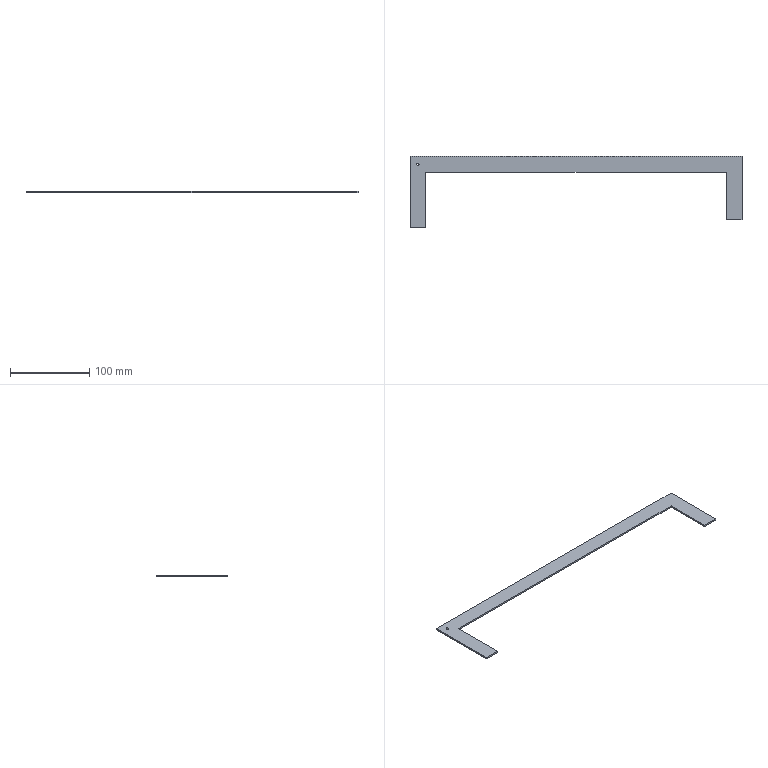Part | STEP file | Trunking Spacer Plate 2 | 1 solid | 12 faces | box 420 x 90 x 2 mm | volume 21986 mm3 | plane 10 | cylinder 2 | commonest cylinder face diameters 3 x2
STEP:
#1=CARTESIAN_POINT('',(1021.716,-891.567,-2.));
#2=VERTEX_POINT('',#1);
#3=CARTESIAN_POINT('',(1018.716,-891.567,-2.));
#4=VERTEX_POINT('',#3);
#5=CARTESIAN_POINT('',(1020.216,-891.567,-2.));
#6=DIRECTION('',(0.,0.,-1.));
#7=DIRECTION('',(1.,0.,0.));
#8=AXIS2_PLACEMENT_3D('',#5,#6,#7);
#9=CIRCLE('',#8,1.5);
#10=EDGE_CURVE('',#2,#4,#9,.T.);
#11=ORIENTED_EDGE('',*,*,#10,.T.);
#12=CARTESIAN_POINT('',(1018.716,-891.567,0.));
#13=VERTEX_POINT('',#12);
#14=CARTESIAN_POINT('',(1018.716,-891.567,-2.));
#15=DIRECTION('',(0.,0.,1.));
#16=VECTOR('',#15,1000.);
#17=LINE('',#14,#16);
#18=EDGE_CURVE('',#4,#13,#17,.T.);
#19=ORIENTED_EDGE('',*,*,#18,.T.);
#20=CARTESIAN_POINT('',(1021.716,-891.567,0.));
#21=VERTEX_POINT('',#20);
#22=CARTESIAN_POINT('',(1020.216,-891.567,0.));
#23=DIRECTION('',(0.,0.,-1.));
#24=DIRECTION('',(1.,0.,0.));
#25=AXIS2_PLACEMENT_3D('',#22,#23,#24);
#26=CIRCLE('',#25,1.5);
#27=EDGE_CURVE('',#21,#13,#26,.T.);
#28=ORIENTED_EDGE('',*,*,#27,.F.);
#29=CARTESIAN_POINT('',(1021.716,-891.567,-2.));
#30=DIRECTION('',(0.,0.,1.));
#31=VECTOR('',#30,1000.);
#32=LINE('',#29,#31);
#33=EDGE_CURVE('',#2,#21,#32,.T.);
#34=ORIENTED_EDGE('',*,*,#33,.F.);
#35=EDGE_LOOP('',(#11,#19,#28,#34));
#36=FACE_OUTER_BOUND('',#35,.T.);
#37=CARTESIAN_POINT('',(1020.216,-891.567,-2.));
#38=DIRECTION('',(0.,0.,1.));
#39=DIRECTION('',(1.,0.,0.));
#40=AXIS2_PLACEMENT_3D('',#37,#38,#39);
#41=CYLINDRICAL_SURFACE('',#40,1.5);
#42=ADVANCED_FACE('',(#36),#41,.F.);
#43=ORIENTED_EDGE('',*,*,#10,.F.);
#44=CARTESIAN_POINT('',(1020.216,-891.567,-2.));
#45=DIRECTION('',(0.,0.,-1.));
#46=DIRECTION('',(1.,0.,0.));
#47=AXIS2_PLACEMENT_3D('',#44,#45,#46);
#48=CIRCLE('',#47,1.5);
#49=EDGE_CURVE('',#4,#2,#48,.T.);
#50=ORIENTED_EDGE('',*,*,#49,.F.);
#51=EDGE_LOOP('',(#43,#50));
#52=FACE_BOUND('',#51,.T.);
#53=CARTESIAN_POINT('',(1410.216,-961.567,-2.));
#54=VERTEX_POINT('',#53);
#55=CARTESIAN_POINT('',(1430.216,-961.567,-2.));
#56=VERTEX_POINT('',#55);
#57=CARTESIAN_POINT('',(0.,-961.567,-2.));
#58=DIRECTION('',(1.,0.,0.));
#59=VECTOR('',#58,1000.);
#60=LINE('',#57,#59);
#61=EDGE_CURVE('',#54,#56,#60,.T.);
#62=ORIENTED_EDGE('',*,*,#61,.F.);
#63=CARTESIAN_POINT('',(1410.216,-901.567,-2.));
#64=VERTEX_POINT('',#63);
#65=CARTESIAN_POINT('',(1410.216,0.,-2.));
#66=DIRECTION('',(0.,-1.,0.));
#67=VECTOR('',#66,1000.);
#68=LINE('',#65,#67);
#69=EDGE_CURVE('',#64,#54,#68,.T.);
#70=ORIENTED_EDGE('',*,*,#69,.F.);
#71=CARTESIAN_POINT('',(1030.216,-901.567,-2.));
#72=VERTEX_POINT('',#71);
#73=CARTESIAN_POINT('',(0.,-901.567,-2.));
#74=DIRECTION('',(1.,0.,0.));
#75=VECTOR('',#74,1000.);
#76=LINE('',#73,#75);
#77=EDGE_CURVE('',#72,#64,#76,.T.);
#78=ORIENTED_EDGE('',*,*,#77,.F.);
#79=CARTESIAN_POINT('',(1030.216,-971.567,-2.));
#80=VERTEX_POINT('',#79);
#81=CARTESIAN_POINT('',(1030.216,0.,-2.));
#82=DIRECTION('',(0.,1.,0.));
#83=VECTOR('',#82,1000.);
#84=LINE('',#81,#83);
#85=EDGE_CURVE('',#80,#72,#84,.T.);
#86=ORIENTED_EDGE('',*,*,#85,.F.);
#87=CARTESIAN_POINT('',(1010.216,-971.567,-2.));
#88=VERTEX_POINT('',#87);
#89=CARTESIAN_POINT('',(0.,-971.567,-2.));
#90=DIRECTION('',(1.,0.,0.));
#91=VECTOR('',#90,1000.);
#92=LINE('',#89,#91);
#93=EDGE_CURVE('',#88,#80,#92,.T.);
#94=ORIENTED_EDGE('',*,*,#93,.F.);
#95=CARTESIAN_POINT('',(1010.216,-881.567,-2.));
#96=VERTEX_POINT('',#95);
#97=CARTESIAN_POINT('',(1010.216,0.,-2.));
#98=DIRECTION('',(0.,-1.,0.));
#99=VECTOR('',#98,1000.);
#100=LINE('',#97,#99);
#101=EDGE_CURVE('',#96,#88,#100,.T.);
#102=ORIENTED_EDGE('',*,*,#101,.F.);
#103=CARTESIAN_POINT('',(1430.216,-881.567,-2.));
#104=VERTEX_POINT('',#103);
#105=CARTESIAN_POINT('',(0.,-881.567,-2.));
#106=DIRECTION('',(-1.,0.,0.));
#107=VECTOR('',#106,1000.);
#108=LINE('',#105,#107);
#109=EDGE_CURVE('',#104,#96,#108,.T.);
#110=ORIENTED_EDGE('',*,*,#109,.F.);
#111=CARTESIAN_POINT('',(1430.216,0.,-2.));
#112=DIRECTION('',(0.,1.,0.));
#113=VECTOR('',#112,1000.);
#114=LINE('',#111,#113);
#115=EDGE_CURVE('',#56,#104,#114,.T.);
#116=ORIENTED_EDGE('',*,*,#115,.F.);
#117=EDGE_LOOP('',(#62,#70,#78,#86,#94,#102,#110,#116));
#118=FACE_OUTER_BOUND('',#117,.T.);
#119=CARTESIAN_POINT('',(0.,0.,-2.));
#120=DIRECTION('',(0.,0.,1.));
#121=DIRECTION('',(1.,0.,0.));
#122=AXIS2_PLACEMENT_3D('',#119,#120,#121);
#123=PLANE('',#122);
#124=ADVANCED_FACE('',(#52,#118),#123,.F.);
#125=ORIENTED_EDGE('',*,*,#18,.F.);
#126=ORIENTED_EDGE('',*,*,#49,.T.);
#127=ORIENTED_EDGE('',*,*,#33,.T.);
#128=CARTESIAN_POINT('',(1020.216,-891.567,0.));
#129=DIRECTION('',(0.,0.,-1.));
#130=DIRECTION('',(1.,0.,0.));
#131=AXIS2_PLACEMENT_3D('',#128,#129,#130);
#132=CIRCLE('',#131,1.5);
#133=EDGE_CURVE('',#13,#21,#132,.T.);
#134=ORIENTED_EDGE('',*,*,#133,.F.);
#135=EDGE_LOOP('',(#125,#126,#127,#134));
#136=FACE_OUTER_BOUND('',#135,.T.);
#137=CARTESIAN_POINT('',(1020.216,-891.567,-2.));
#138=DIRECTION('',(0.,0.,1.));
#139=DIRECTION('',(1.,0.,0.));
#140=AXIS2_PLACEMENT_3D('',#137,#138,#139);
#141=CYLINDRICAL_SURFACE('',#140,1.5);
#142=ADVANCED_FACE('',(#136),#141,.F.);
#143=CARTESIAN_POINT('',(1430.216,-881.567,0.));
#144=VERTEX_POINT('',#143);
#145=CARTESIAN_POINT('',(1430.216,-881.567,-2.));
#146=DIRECTION('',(0.,0.,1.));
#147=VECTOR('',#146,1000.);
#148=LINE('',#145,#147);
#149=EDGE_CURVE('',#104,#144,#148,.T.);
#150=ORIENTED_EDGE('',*,*,#149,.T.);
#151=CARTESIAN_POINT('',(1430.216,-961.567,0.));
#152=VERTEX_POINT('',#151);
#153=CARTESIAN_POINT('',(1430.216,-881.567,0.));
#154=DIRECTION('',(0.,-1.,0.));
#155=VECTOR('',#154,1000.);
#156=LINE('',#153,#155);
#157=EDGE_CURVE('',#144,#152,#156,.T.);
#158=ORIENTED_EDGE('',*,*,#157,.T.);
#159=CARTESIAN_POINT('',(1430.216,-961.567,-2.));
#160=DIRECTION('',(0.,0.,-1.));
#161=VECTOR('',#160,1000.);
#162=LINE('',#159,#161);
#163=EDGE_CURVE('',#152,#56,#162,.T.);
#164=ORIENTED_EDGE('',*,*,#163,.T.);
#165=ORIENTED_EDGE('',*,*,#115,.T.);
#166=EDGE_LOOP('',(#150,#158,#164,#165));
#167=FACE_OUTER_BOUND('',#166,.T.);
#168=CARTESIAN_POINT('',(1430.216,-881.567,-2.));
#169=DIRECTION('',(1.,0.,0.));
#170=DIRECTION('',(0.,1.,0.));
#171=AXIS2_PLACEMENT_3D('',#168,#169,#170);
#172=PLANE('',#171);
#173=ADVANCED_FACE('',(#167),#172,.T.);
#174=CARTESIAN_POINT('',(1410.216,-961.567,0.));
#175=VERTEX_POINT('',#174);
#176=CARTESIAN_POINT('',(1010.216,-961.567,0.));
#177=DIRECTION('',(1.,0.,0.));
#178=VECTOR('',#177,1000.);
#179=LINE('',#176,#178);
#180=EDGE_CURVE('',#175,#152,#179,.T.);
#181=ORIENTED_EDGE('',*,*,#180,.F.);
#182=CARTESIAN_POINT('',(1410.216,-961.567,-10.));
#183=DIRECTION('',(0.,0.,1.));
#184=VECTOR('',#183,1000.);
#185=LINE('',#182,#184);
#186=EDGE_CURVE('',#54,#175,#185,.T.);
#187=ORIENTED_EDGE('',*,*,#186,.F.);
#188=ORIENTED_EDGE('',*,*,#61,.T.);
#189=ORIENTED_EDGE('',*,*,#163,.F.);
#190=EDGE_LOOP('',(#181,#187,#188,#189));
#191=FACE_OUTER_BOUND('',#190,.T.);
#192=CARTESIAN_POINT('',(1010.216,-961.567,-10.));
#193=DIRECTION('',(0.,1.,0.));
#194=DIRECTION('',(0.,0.,1.));
#195=AXIS2_PLACEMENT_3D('',#192,#193,#194);
#196=PLANE('',#195);
#197=ADVANCED_FACE('',(#191),#196,.F.);
#198=ORIENTED_EDGE('',*,*,#186,.T.);
#199=CARTESIAN_POINT('',(1410.216,-901.567,0.));
#200=VERTEX_POINT('',#199);
#201=CARTESIAN_POINT('',(1410.216,-901.567,0.));
#202=DIRECTION('',(0.,-1.,0.));
#203=VECTOR('',#202,1000.);
#204=LINE('',#201,#203);
#205=EDGE_CURVE('',#200,#175,#204,.T.);
#206=ORIENTED_EDGE('',*,*,#205,.F.);
#207=CARTESIAN_POINT('',(1410.216,-901.567,-2.));
#208=DIRECTION('',(0.,0.,1.));
#209=VECTOR('',#208,1000.);
#210=LINE('',#207,#209);
#211=EDGE_CURVE('',#64,#200,#210,.T.);
#212=ORIENTED_EDGE('',*,*,#211,.F.);
#213=ORIENTED_EDGE('',*,*,#69,.T.);
#214=EDGE_LOOP('',(#198,#206,#212,#213));
#215=FACE_OUTER_BOUND('',#214,.T.);
#216=CARTESIAN_POINT('',(1410.216,-901.567,-2.));
#217=DIRECTION('',(1.,0.,0.));
#218=DIRECTION('',(0.,0.,-1.));
#219=AXIS2_PLACEMENT_3D('',#216,#217,#218);
#220=PLANE('',#219);
#221=ADVANCED_FACE('',(#215),#220,.F.);
#222=CARTESIAN_POINT('',(1030.216,-901.567,0.));
#223=VERTEX_POINT('',#222);
#224=CARTESIAN_POINT('',(1030.216,-901.567,-2.));
#225=DIRECTION('',(0.,0.,1.));
#226=VECTOR('',#225,1000.);
#227=LINE('',#224,#226);
#228=EDGE_CURVE('',#72,#223,#227,.T.);
#229=ORIENTED_EDGE('',*,*,#228,.F.);
#230=ORIENTED_EDGE('',*,*,#77,.T.);
#231=ORIENTED_EDGE('',*,*,#211,.T.);
#232=CARTESIAN_POINT('',(1030.216,-901.567,0.));
#233=DIRECTION('',(1.,0.,0.));
#234=VECTOR('',#233,1000.);
#235=LINE('',#232,#234);
#236=EDGE_CURVE('',#223,#200,#235,.T.);
#237=ORIENTED_EDGE('',*,*,#236,.F.);
#238=EDGE_LOOP('',(#229,#230,#231,#237));
#239=FACE_OUTER_BOUND('',#238,.T.);
#240=CARTESIAN_POINT('',(1030.216,-901.567,-2.));
#241=DIRECTION('',(0.,1.,0.));
#242=DIRECTION('',(0.,0.,1.));
#243=AXIS2_PLACEMENT_3D('',#240,#241,#242);
#244=PLANE('',#243);
#245=ADVANCED_FACE('',(#239),#244,.F.);
#246=CARTESIAN_POINT('',(1030.216,-971.567,0.));
#247=VERTEX_POINT('',#246);
#248=CARTESIAN_POINT('',(1030.216,-971.567,-2.));
#249=DIRECTION('',(0.,0.,1.));
#250=VECTOR('',#249,1000.);
#251=LINE('',#248,#250);
#252=EDGE_CURVE('',#80,#247,#251,.T.);
#253=ORIENTED_EDGE('',*,*,#252,.F.);
#254=ORIENTED_EDGE('',*,*,#85,.T.);
#255=ORIENTED_EDGE('',*,*,#228,.T.);
#256=CARTESIAN_POINT('',(1030.216,-901.567,0.));
#257=DIRECTION('',(0.,1.,0.));
#258=VECTOR('',#257,1000.);
#259=LINE('',#256,#258);
#260=EDGE_CURVE('',#247,#223,#259,.T.);
#261=ORIENTED_EDGE('',*,*,#260,.F.);
#262=EDGE_LOOP('',(#253,#254,#255,#261));
#263=FACE_OUTER_BOUND('',#262,.T.);
#264=CARTESIAN_POINT('',(1030.216,-901.567,-2.));
#265=DIRECTION('',(-1.,0.,0.));
#266=DIRECTION('',(0.,0.,1.));
#267=AXIS2_PLACEMENT_3D('',#264,#265,#266);
#268=PLANE('',#267);
#269=ADVANCED_FACE('',(#263),#268,.F.);
#270=CARTESIAN_POINT('',(1010.216,-971.567,0.));
#271=VERTEX_POINT('',#270);
#272=CARTESIAN_POINT('',(0.,-971.567,0.));
#273=DIRECTION('',(-1.,0.,0.));
#274=VECTOR('',#273,1000.);
#275=LINE('',#272,#274);
#276=EDGE_CURVE('',#247,#271,#275,.T.);
#277=ORIENTED_EDGE('',*,*,#276,.T.);
#278=CARTESIAN_POINT('',(1010.216,-971.567,0.));
#279=DIRECTION('',(0.,0.,-1.));
#280=VECTOR('',#279,1000.);
#281=LINE('',#278,#280);
#282=EDGE_CURVE('',#271,#88,#281,.T.);
#283=ORIENTED_EDGE('',*,*,#282,.T.);
#284=ORIENTED_EDGE('',*,*,#93,.T.);
#285=ORIENTED_EDGE('',*,*,#252,.T.);
#286=EDGE_LOOP('',(#277,#283,#284,#285));
#287=FACE_OUTER_BOUND('',#286,.T.);
#288=CARTESIAN_POINT('',(0.,-971.567,0.));
#289=DIRECTION('',(0.,-1.,0.));
#290=DIRECTION('',(0.,0.,-1.));
#291=AXIS2_PLACEMENT_3D('',#288,#289,#290);
#292=PLANE('',#291);
#293=ADVANCED_FACE('',(#287),#292,.T.);
#294=CARTESIAN_POINT('',(1010.216,-881.567,0.));
#295=VERTEX_POINT('',#294);
#296=CARTESIAN_POINT('',(1010.216,-881.567,0.));
#297=DIRECTION('',(0.,1.,0.));
#298=VECTOR('',#297,1000.);
#299=LINE('',#296,#298);
#300=EDGE_CURVE('',#271,#295,#299,.T.);
#301=ORIENTED_EDGE('',*,*,#300,.T.);
#302=CARTESIAN_POINT('',(1010.216,-881.567,-2.));
#303=DIRECTION('',(0.,0.,-1.));
#304=VECTOR('',#303,1000.);
#305=LINE('',#302,#304);
#306=EDGE_CURVE('',#295,#96,#305,.T.);
#307=ORIENTED_EDGE('',*,*,#306,.T.);
#308=ORIENTED_EDGE('',*,*,#101,.T.);
#309=ORIENTED_EDGE('',*,*,#282,.F.);
#310=EDGE_LOOP('',(#301,#307,#308,#309));
#311=FACE_OUTER_BOUND('',#310,.T.);
#312=CARTESIAN_POINT('',(1010.216,-881.567,-2.));
#313=DIRECTION('',(-1.,0.,0.));
#314=DIRECTION('',(0.,-1.,0.));
#315=AXIS2_PLACEMENT_3D('',#312,#313,#314);
#316=PLANE('',#315);
#317=ADVANCED_FACE('',(#311),#316,.T.);
#318=ORIENTED_EDGE('',*,*,#109,.T.);
#319=ORIENTED_EDGE('',*,*,#306,.F.);
#320=CARTESIAN_POINT('',(1010.216,-881.567,0.));
#321=DIRECTION('',(1.,0.,0.));
#322=VECTOR('',#321,1000.);
#323=LINE('',#320,#322);
#324=EDGE_CURVE('',#295,#144,#323,.T.);
#325=ORIENTED_EDGE('',*,*,#324,.T.);
#326=ORIENTED_EDGE('',*,*,#149,.F.);
#327=EDGE_LOOP('',(#318,#319,#325,#326));
#328=FACE_OUTER_BOUND('',#327,.T.);
#329=CARTESIAN_POINT('',(1010.216,-881.567,-2.));
#330=DIRECTION('',(0.,1.,0.));
#331=DIRECTION('',(0.,0.,1.));
#332=AXIS2_PLACEMENT_3D('',#329,#330,#331);
#333=PLANE('',#332);
#334=ADVANCED_FACE('',(#328),#333,.T.);
#335=ORIENTED_EDGE('',*,*,#27,.T.);
#336=ORIENTED_EDGE('',*,*,#133,.T.);
#337=EDGE_LOOP('',(#335,#336));
#338=FACE_BOUND('',#337,.T.);
#339=ORIENTED_EDGE('',*,*,#236,.T.);
#340=ORIENTED_EDGE('',*,*,#205,.T.);
#341=ORIENTED_EDGE('',*,*,#180,.T.);
#342=ORIENTED_EDGE('',*,*,#157,.F.);
#343=ORIENTED_EDGE('',*,*,#324,.F.);
#344=ORIENTED_EDGE('',*,*,#300,.F.);
#345=ORIENTED_EDGE('',*,*,#276,.F.);
#346=ORIENTED_EDGE('',*,*,#260,.T.);
#347=EDGE_LOOP('',(#339,#340,#341,#342,#343,#344,#345,#346));
#348=FACE_OUTER_BOUND('',#347,.T.);
#349=CARTESIAN_POINT('',(0.,0.,0.));
#350=DIRECTION('',(0.,0.,1.));
#351=DIRECTION('',(1.,0.,0.));
#352=AXIS2_PLACEMENT_3D('',#349,#350,#351);
#353=PLANE('',#352);
#354=ADVANCED_FACE('',(#338,#348),#353,.T.);
#355=CLOSED_SHELL('',(#42,#124,#142,#173,#197,#221,#245,#269,#293,#317,#334,#354));
#356=MANIFOLD_SOLID_BREP('',#355);
#357=CARTESIAN_POINT('',(0.,0.,0.));
#358=DIRECTION('',(0.,0.,1.));
#359=DIRECTION('',(1.,0.,0.));
#360=AXIS2_PLACEMENT_3D('',#357,#358,#359);
#361=(LENGTH_UNIT()NAMED_UNIT(*)SI_UNIT(.MILLI.,.METRE.));
#362=UNCERTAINTY_MEASURE_WITH_UNIT(LENGTH_MEASURE(0.00001),#361,'','');
#363=(NAMED_UNIT(*)PLANE_ANGLE_UNIT()SI_UNIT($,.RADIAN.));
#364=(NAMED_UNIT(*)SI_UNIT($,.STERADIAN.)SOLID_ANGLE_UNIT());
#365=(GEOMETRIC_REPRESENTATION_CONTEXT(3)GLOBAL_UNCERTAINTY_ASSIGNED_CONTEXT((#362))GLOBAL_UNIT_ASSIGNED_CONTEXT((#361,#363,#364))REPRESENTATION_CONTEXT('',''));
#366=ADVANCED_BREP_SHAPE_REPRESENTATION('',(#356,#360),#365);